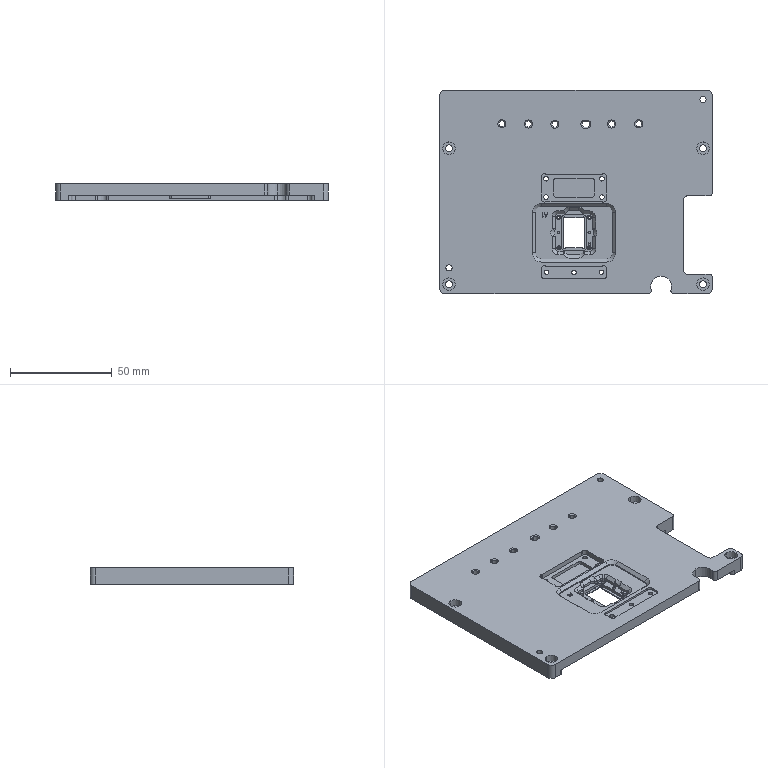NC program | NX | posted with a generic post | part box 134 x 100 x 8 mm
Lines 5752 to 6609 of 16793:
(ZLEVEL_PROFILE_COPY_COPY_COPY_1_COPY_COPY_1_COPY_COPY_COPY_1_COPY_COPY_COPY , )
N11424 T18 M6
N11426 G54
N11428 G17 G0 G90 X-14.95 Y-1.854 S9500 M3
N11430 G43 Z30. H18
N11432 Z-0.177
N11434 G94 G1 X-15.4 Y-2.113 F1000.
N11436 G3 X-15.55 Y-2.373 R0.3
N11438 G1 Y-2.49 F1100.
N11440 G2 X-15.685 Y-3.174 R1.8
N11442 G3 X-15.418 Y-3.432 R0.2
N11444 G2 X-14.802 Y-3.3 R1.5
N11446 G1 X-14.629
N11448 G3 X-14.369 Y-3.15 R0.3
N11450 G1 X-14.109 Y-2.7
N11452 G0 X-14.95 Y-1.854 Z-0.354
N11454 G1 X-15.4 Y-2.113 F1000.
N11456 G3 X-15.55 Y-2.373 R0.3
N11458 G1 Y-2.49 F1100.
N11460 G2 X-15.685 Y-3.174 R1.8
N11462 G3 X-15.418 Y-3.432 R0.2
N11464 G2 X-14.802 Y-3.3 R1.5
N11466 G1 X-14.629
N11468 G3 X-14.369 Y-3.15 R0.3
N11470 G1 X-14.109 Y-2.7
N11472 G0 X-14.95 Y-1.854 Z-0.515
N11474 G1 X-15.4 Y-2.113 F1000.
N11476 G3 X-15.55 Y-2.373 R0.3
N11478 G1 Y-2.49 F1100.
N11480 G2 X-15.685 Y-3.174 R1.8
N11482 G3 X-15.418 Y-3.432 R0.2
N11484 G2 X-14.802 Y-3.3 R1.5
N11486 G1 X-14.629
N11488 G3 X-14.369 Y-3.15 R0.3
N11490 G1 X-14.109 Y-2.7
N11492 G0 X-14.95 Y-1.854 Z-0.677
N11494 G1 X-15.4 Y-2.113 F1000.
N11496 G3 X-15.55 Y-2.373 R0.3
N11498 G1 Y-2.49 F1100.
N11500 G2 X-15.685 Y-3.174 R1.8
N11502 G3 X-15.418 Y-3.432 R0.2
N11504 G2 X-14.802 Y-3.3 R1.5
N11506 G1 X-14.629
N11508 G3 X-14.369 Y-3.15 R0.3
N11510 G1 X-14.109 Y-2.7
N11512 G0 X-14.95 Y-1.854 Z-0.838
N11514 G1 X-15.4 Y-2.113 F1000.
N11516 G3 X-15.55 Y-2.373 R0.3
N11518 G1 Y-2.49 F1100.
N11520 G2 X-15.685 Y-3.174 R1.8
N11522 G3 X-15.418 Y-3.432 R0.2
N11524 G2 X-14.802 Y-3.3 R1.5
N11526 G1 X-14.629
N11528 G3 X-14.369 Y-3.15 R0.3
N11530 G1 X-14.109 Y-2.7
N11532 G0 X-14.95 Y-1.854 Z-1.
N11534 G1 X-15.4 Y-2.113 F1000.
N11536 G3 X-15.55 Y-2.373 R0.3
N11538 G1 Y-2.49 F1100.
N11540 G2 X-15.685 Y-3.174 R1.8
N11542 G3 X-15.418 Y-3.432 R0.2
N11544 G2 X-14.802 Y-3.3 R1.5
N11546 G1 X-14.629
N11548 G3 X-14.369 Y-3.15 R0.3
N11550 G1 X-14.109 Y-2.7
N11552 G0 X-14.95 Y-1.854 Z-1.177
N11554 G1 X-15.4 Y-2.113 F1000.
N11556 G3 X-15.55 Y-2.373 R0.3
N11558 G1 Y-2.49 F1100.
N11560 G2 X-15.685 Y-3.174 R1.8
N11562 G3 X-15.418 Y-3.432 R0.2
N11564 G2 X-14.802 Y-3.3 R1.5
N11566 G1 X-14.629
N11568 G3 X-14.369 Y-3.15 R0.3
N11570 G1 X-14.109 Y-2.7
N11572 G0 X-14.95 Y-1.854 Z-1.354
N11574 G1 X-15.4 Y-2.113 F1000.
N11576 G3 X-15.55 Y-2.373 R0.3
N11578 G1 Y-2.49 F1100.
N11580 G2 X-15.685 Y-3.174 R1.8
N11582 G3 X-15.418 Y-3.432 R0.2
N11584 G2 X-14.802 Y-3.3 R1.5
N11586 G1 X-14.629
N11588 G3 X-14.369 Y-3.15 R0.3
N11590 G1 X-14.109 Y-2.7
N11592 G0 X-14.95 Y-1.854 Z-1.544
N11594 G1 X-15.4 Y-2.113 F1000.
N11596 G3 X-15.55 Y-2.373 R0.3
N11598 G1 Y-2.49 F1100.
N11600 G2 X-15.685 Y-3.174 R1.8
N11602 G3 X-15.418 Y-3.432 R0.2
N11604 G2 X-14.802 Y-3.3 R1.5
N11606 G1 X-14.629
N11608 G3 X-14.369 Y-3.15 R0.3
N11610 G1 X-14.109 Y-2.7
N11612 G0 X-14.95 Y-1.854 Z-1.794
N11614 G1 X-15.4 Y-2.113 F1000.
N11616 G3 X-15.55 Y-2.373 R0.3
N11618 G1 Y-2.49 F1100.
N11620 G2 X-15.685 Y-3.174 R1.8
N11622 G3 X-15.418 Y-3.432 R0.2
N11624 G2 X-14.802 Y-3.3 R1.5
N11626 G1 X-14.629
N11628 G3 X-14.369 Y-3.15 R0.3
N11630 G1 X-14.109 Y-2.7
N11632 G0 X-14.95 Y-1.854 Z-2.
N11634 G1 X-15.4 Y-2.113 F1000.
N11636 G3 X-15.55 Y-2.373 R0.3
N11638 G1 Y-2.49 F1100.
N11640 G2 X-15.685 Y-3.174 R1.8
N11642 G3 X-15.418 Y-3.432 R0.2
N11644 G2 X-14.802 Y-3.3 R1.5
N11646 G1 X-14.629
N11648 G3 X-14.369 Y-3.15 R0.3
N11650 G1 X-14.109 Y-2.7
N11652 G0 X-14.95 Y-1.854 Z-2.1
N11654 G1 X-15.4 Y-2.113 F1000.
N11656 G3 X-15.55 Y-2.373 R0.3
N11658 G1 Y-2.49 F1100.
N11660 G2 X-15.685 Y-3.174 R1.8
N11662 G3 X-15.418 Y-3.432 R0.2
N11664 G2 X-14.802 Y-3.3 R1.5
N11666 G1 X-14.629
N11668 G3 X-14.369 Y-3.15 R0.3
N11670 G1 X-14.109 Y-2.7
N11672 G0 X-14.95 Y-1.854 Z-2.267
N11674 G1 X-15.4 Y-2.113 F1000.
N11676 G3 X-15.55 Y-2.373 R0.3
N11678 G1 Y-2.49 F1100.
N11680 G2 X-15.685 Y-3.174 R1.8
N11682 G3 X-15.418 Y-3.432 R0.2
N11684 G2 X-14.802 Y-3.3 R1.5
N11686 G1 X-14.629
N11688 G3 X-14.369 Y-3.15 R0.3
N11690 G1 X-14.109 Y-2.7
N11692 G0 X-14.95 Y-1.854 Z-2.433
N11694 G1 X-15.4 Y-2.113 F1000.
N11696 G3 X-15.55 Y-2.373 R0.3
N11698 G1 Y-2.49 F1100.
N11700 G2 X-15.685 Y-3.174 R1.8
N11702 G3 X-15.418 Y-3.432 R0.2
N11704 G2 X-14.802 Y-3.3 R1.5
N11706 G1 X-14.629
N11708 G3 X-14.369 Y-3.15 R0.3
N11710 G1 X-14.109 Y-2.7
N11712 G0 X-14.95 Y-1.854 Z-2.6
N11714 G1 X-15.4 Y-2.113 F1000.
N11716 G3 X-15.55 Y-2.373 R0.3
N11718 G1 Y-2.49 F1100.
N11720 G2 X-15.685 Y-3.174 R1.8
N11722 G3 X-15.418 Y-3.432 R0.2
N11724 G2 X-14.802 Y-3.3 R1.5
N11726 G1 X-14.629
N11728 G3 X-14.369 Y-3.15 R0.3
N11730 G1 X-14.109 Y-2.7
N11732 G0 Z30.
N11734 X12.108
N11736 Z-0.177
N11738 G1 X12.368 Y-3.15 F1000.
N11740 G3 X12.627 Y-3.3 R0.3
N11742 G1 X12.74 F1100.
N11744 G2 X13.424 Y-3.435 R1.8
N11746 G3 X13.685 Y-3.174 R0.2
N11748 G2 X13.55 Y-2.49 R1.8
N11750 G1 Y-2.376
N11752 G3 X13.4 Y-2.116 R0.3
N11754 G1 X12.95 Y-1.857
N11756 G0 X12.108 Y-2.7 Z-0.354
N11758 G1 X12.367 Y-3.15 F1000.
N11760 G3 X12.627 Y-3.3 R0.3
N11762 G1 X12.74 F1100.
N11764 G2 X13.424 Y-3.435 R1.8
N11766 G3 X13.685 Y-3.174 R0.2
N11768 G2 X13.55 Y-2.49 R1.8
N11770 G1 Y-2.376
N11772 G3 X13.4 Y-2.116 R0.3
N11774 G1 X12.95 Y-1.856
N11776 G0 X12.108 Y-2.7 Z-0.515
N11778 G1 X12.367 Y-3.15 F1000.
N11780 G3 X12.627 Y-3.3 R0.3
N11782 G1 X12.74 F1100.
N11784 G2 X13.424 Y-3.435 R1.8
N11786 G3 X13.685 Y-3.174 R0.2
N11788 G2 X13.55 Y-2.49 R1.8
N11790 G1 Y-2.375
N11792 G3 X13.4 Y-2.116 R0.3
N11794 G1 X12.95 Y-1.856
N11796 G0 X12.107 Y-2.7 Z-0.677
N11798 G1 X12.367 Y-3.15 F1000.
N11800 G3 X12.627 Y-3.3 R0.3
N11802 G1 X12.74 F1100.
N11804 G2 X13.424 Y-3.435 R1.8
N11806 G3 X13.685 Y-3.174 R0.2
N11808 G2 X13.55 Y-2.49 R1.8
N11810 G1 Y-2.375
N11812 G3 X13.4 Y-2.115 R0.3
N11814 G1 X12.95 Y-1.855
N11816 G0 X12.107 Y-2.7 Z-0.838
N11818 G1 X12.367 Y-3.15 F1000.
N11820 G3 X12.627 Y-3.3 R0.3
N11822 G1 X12.74 F1100.
N11824 G2 X13.424 Y-3.435 R1.8
N11826 G3 X13.685 Y-3.174 R0.2
N11828 G2 X13.55 Y-2.49 R1.8
N11830 G1 Y-2.375
N11832 G3 X13.4 Y-2.115 R0.3
N11834 G1 X12.95 Y-1.855
N11836 G0 X12.107 Y-2.7 Z-1.
N11838 G1 X12.367 Y-3.15 F1000.
N11840 G3 X12.627 Y-3.3 R0.3
N11842 G1 X12.74 F1100.
N11844 G2 X13.424 Y-3.435 R1.8
N11846 G3 X13.685 Y-3.174 R0.2
N11848 G2 X13.55 Y-2.49 R1.8
N11850 G1 Y-2.374
N11852 G3 X13.4 Y-2.114 R0.3
N11854 G1 X12.95 Y-1.855
N11856 G0 X12.107 Y-2.7 Z-1.177
N11858 G1 X12.367 Y-3.15 F1000.
N11860 G3 X12.627 Y-3.3 R0.3
N11862 G1 X12.74 F1100.
N11864 G2 X13.424 Y-3.435 R1.8
N11866 G3 X13.685 Y-3.174 R0.2
N11868 G2 X13.55 Y-2.49 R1.8
N11870 G1 Y-2.374
N11872 G3 X13.4 Y-2.114 R0.3
N11874 G1 X12.95 Y-1.854
N11876 G0 X12.107 Y-2.7 Z-1.354
N11878 G1 X12.367 Y-3.15 F1000.
N11880 G3 X12.627 Y-3.3 R0.3
N11882 G1 X12.74 F1100.
N11884 G2 X13.424 Y-3.435 R1.8
N11886 G3 X13.685 Y-3.174 R0.2
N11888 G2 X13.55 Y-2.49 R1.8
N11890 G1 Y-2.373
N11892 G3 X13.4 Y-2.113 R0.3
N11894 G1 X12.95 Y-1.854
N11896 G0 X12.107 Y-2.7 Z-1.544
N11898 G1 X12.367 Y-3.15 F1000.
N11900 G3 X12.627 Y-3.3 R0.3
N11902 G1 X12.74 F1100.
N11904 G2 X13.424 Y-3.435 R1.8
N11906 G3 X13.685 Y-3.174 R0.2
N11908 G2 X13.55 Y-2.49 R1.8
N11910 G1 Y-2.373
N11912 G3 X13.4 Y-2.113 R0.3
N11914 G1 X12.95 Y-1.853
N11916 G0 X12.107 Y-2.7 Z-1.794
N11918 G1 X12.367 Y-3.15 F1000.
N11920 G3 X12.626 Y-3.3 R0.3
N11922 G1 X12.74 F1100.
N11924 G2 X13.424 Y-3.435 R1.8
N11926 G3 X13.685 Y-3.174 R0.2
N11928 G2 X13.55 Y-2.49 R1.8
N11930 G1 Y-2.372
N11932 G3 X13.4 Y-2.112 R0.3
N11934 G1 X12.95 Y-1.853
N11936 G0 X12.107 Y-2.7 Z-2.
N11938 G1 X12.367 Y-3.15 F1000.
N11940 G3 X12.626 Y-3.3 R0.3
N11942 G1 X12.74 F1100.
N11944 G2 X13.424 Y-3.435 R1.8
N11946 G3 X13.685 Y-3.174 R0.2
N11948 G2 X13.55 Y-2.49 R1.8
N11950 G1 Y-2.372
N11952 G3 X13.4 Y-2.112 R0.3
N11954 G1 X12.95 Y-1.852
N11956 G0 X12.107 Y-2.7 Z-2.1
N11958 G1 X12.366 Y-3.15 F1000.
N11960 G3 X12.626 Y-3.3 R0.3
N11962 G1 X12.74 F1100.
N11964 G2 X13.424 Y-3.435 R1.8
N11966 G3 X13.685 Y-3.174 R0.2
N11968 G2 X13.55 Y-2.49 R1.8
N11970 G1 Y-2.371
N11972 G3 X13.4 Y-2.112 R0.3
N11974 G1 X12.95 Y-1.852
N11976 G0 X12.107 Y-2.7 Z-2.267
N11978 G1 X12.366 Y-3.15 F1000.
N11980 G3 X12.626 Y-3.3 R0.3
N11982 G1 X12.74 F1100.
N11984 G2 X13.424 Y-3.435 R1.8
N11986 G3 X13.685 Y-3.174 R0.2
N11988 G2 X13.55 Y-2.49 R1.8
N11990 G1 Y-2.371
N11992 G3 X13.4 Y-2.111 R0.3
N11994 G1 X12.95 Y-1.851
N11996 G0 X12.106 Y-2.7 Z-2.433
N11998 G1 X12.366 Y-3.15 F1000.
N12000 G3 X12.626 Y-3.3 R0.3
N12002 G1 X12.74 F1100.
N12004 G2 X13.424 Y-3.435 R1.8
N12006 G3 X13.685 Y-3.174 R0.2
N12008 G2 X13.55 Y-2.49 R1.8
N12010 G1 Y-2.371
N12012 G3 X13.4 Y-2.111 R0.3
N12014 G1 X12.95 Y-1.851
N12016 G0 X12.106 Y-2.7 Z-2.6
N12018 G1 X12.366 Y-3.15 F1000.
N12020 G3 X12.626 Y-3.3 R0.3
N12022 G1 X12.74 F1100.
N12024 G2 X13.424 Y-3.435 R1.8
N12026 G3 X13.685 Y-3.174 R0.2
N12028 G2 X13.55 Y-2.49 R1.8
N12030 G1 Y-2.37
N12032 G3 X13.4 Y-2.11 R0.3
N12034 G1 X12.95 Y-1.85
N12036 G0 Z30.
N12038 Y5.858
N12040 Z-0.177
N12042 G1 X13.4 Y6.118 F1000.
N12044 G3 X13.55 Y6.378 R0.3
N12046 G1 Y6.49 F1100.
N12048 G2 X13.685 Y7.174 R1.8
N12050 G3 X13.424 Y7.435 R0.2
N12052 G2 X12.74 Y7.3 R1.8
N12054 G1 X12.628
N12056 G3 X12.368 Y7.15 R0.3
N12058 G1 X12.108 Y6.7
N12060 G0 X12.95 Y5.858 Z-0.354
N12062 G1 X13.4 Y6.118 F1000.
N12064 G3 X13.55 Y6.378 R0.3
N12066 G1 Y6.49 F1100.
N12068 G2 X13.685 Y7.174 R1.8
N12070 G3 X13.424 Y7.435 R0.2
N12072 G2 X12.74 Y7.3 R1.8
N12074 G1 X12.628
N12076 G3 X12.368 Y7.15 R0.3
N12078 G1 X12.108 Y6.7
N12080 G0 X12.95 Y5.858 Z-0.515
N12082 G1 X13.4 Y6.118 F1000.
N12084 G3 X13.55 Y6.378 R0.3
N12086 G1 Y6.49 F1100.
N12088 G2 X13.685 Y7.174 R1.8
N12090 G3 X13.424 Y7.435 R0.2
N12092 G2 X12.74 Y7.3 R1.8
N12094 G1 X12.628
N12096 G3 X12.368 Y7.15 R0.3
N12098 G1 X12.108 Y6.7
N12100 G0 X12.95 Y5.858 Z-0.677
N12102 G1 X13.4 Y6.118 F1000.
N12104 G3 X13.55 Y6.377 R0.3
N12106 G1 Y6.49 F1100.
N12108 G2 X13.685 Y7.174 R1.8
N12110 G3 X13.424 Y7.435 R0.2
N12112 G2 X12.74 Y7.3 R1.8
N12114 G1 X12.627
N12116 G3 X12.368 Y7.15 R0.3
N12118 G1 X12.108 Y6.7
N12120 G0 X12.95 Y5.858 Z-0.838
N12122 G1 X13.4 Y6.118 F1000.
N12124 G3 X13.55 Y6.377 R0.3
N12126 G1 Y6.49 F1100.
N12128 G2 X13.685 Y7.174 R1.8
N12130 G3 X13.424 Y7.435 R0.2
N12132 G2 X12.74 Y7.3 R1.8
N12134 G1 X12.627
N12136 G3 X12.368 Y7.15 R0.3
N12138 G1 X12.108 Y6.7
N12140 G0 X12.95 Y5.858 Z-1.
N12142 G1 X13.4 Y6.118 F1000.
N12144 G3 X13.55 Y6.377 R0.3
N12146 G1 Y6.49 F1100.
N12148 G2 X13.685 Y7.174 R1.8
N12150 G3 X13.424 Y7.435 R0.2
N12152 G2 X12.74 Y7.3 R1.8
N12154 G1 X12.627
N12156 G3 X12.368 Y7.15 R0.3
N12158 G1 X12.108 Y6.7
N12160 G0 X12.95 Y5.858 Z-1.177
N12162 G1 X13.4 Y6.117 F1000.
N12164 G3 X13.55 Y6.377 R0.3
N12166 G1 Y6.49 F1100.
N12168 G2 X13.685 Y7.174 R1.8
N12170 G3 X13.424 Y7.435 R0.2
N12172 G2 X12.74 Y7.3 R1.8
N12174 G1 X12.627
N12176 G3 X12.367 Y7.15 R0.3
N12178 G1 X12.108 Y6.7
N12180 G0 X12.95 Y5.858 Z-1.354
N12182 G1 X13.4 Y6.117 F1000.
N12184 G3 X13.55 Y6.377 R0.3
N12186 G1 Y6.49 F1100.
N12188 G2 X13.685 Y7.174 R1.8
N12190 G3 X13.424 Y7.435 R0.2
N12192 G2 X12.74 Y7.3 R1.8
N12194 G1 X12.627
N12196 G3 X12.367 Y7.15 R0.3
N12198 G1 X12.108 Y6.7
N12200 G0 X12.95 Y5.857 Z-1.544
N12202 G1 X13.4 Y6.117 F1000.
N12204 G3 X13.55 Y6.377 R0.3
N12206 G1 Y6.49 F1100.
N12208 G2 X13.685 Y7.174 R1.8
N12210 G3 X13.424 Y7.435 R0.2
N12212 G2 X12.74 Y7.3 R1.8
N12214 G1 X12.627
N12216 G3 X12.367 Y7.15 R0.3
N12218 G1 X12.107 Y6.7
N12220 G0 X12.95 Y5.857 Z-1.794
N12222 G1 X13.4 Y6.117 F1000.
N12224 G3 X13.55 Y6.377 R0.3
N12226 G1 Y6.49 F1100.
N12228 G2 X13.685 Y7.174 R1.8
N12230 G3 X13.424 Y7.435 R0.2
N12232 G2 X12.74 Y7.3 R1.8
N12234 G1 X12.627
N12236 G3 X12.367 Y7.15 R0.3
N12238 G1 X12.107 Y6.7
N12240 G0 X12.95 Y5.857 Z-2.
N12242 G1 X13.4 Y6.117 F1000.
N12244 G3 X13.55 Y6.377 R0.3
N12246 G1 Y6.49 F1100.
N12248 G2 X13.685 Y7.174 R1.8
N12250 G3 X13.424 Y7.435 R0.2
N12252 G2 X12.74 Y7.3 R1.8
N12254 G1 X12.627
N12256 G3 X12.367 Y7.15 R0.3
N12258 G1 X12.107 Y6.7
N12260 G0 X12.95 Y5.857 Z-2.1
N12262 G1 X13.4 Y6.117 F1000.
N12264 G3 X13.55 Y6.377 R0.3
N12266 G1 Y6.49 F1100.
N12268 G2 X13.685 Y7.174 R1.8
N12270 G3 X13.424 Y7.435 R0.2
N12272 G2 X12.74 Y7.3 R1.8
N12274 G1 X12.627
N12276 G3 X12.367 Y7.15 R0.3
N12278 G1 X12.107 Y6.7
N12280 G0 X12.95 Y5.857 Z-2.267
N12282 G1 X13.4 Y6.117 F1000.
N12284 G3 X13.55 Y6.377 R0.3
N12286 G1 Y6.49 F1100.
N12288 G2 X13.685 Y7.174 R1.8
N12290 G3 X13.424 Y7.435 R0.2
N12292 G2 X12.74 Y7.3 R1.8
N12294 G1 X12.627
N12296 G3 X12.367 Y7.15 R0.3
N12298 G1 X12.107 Y6.7
N12300 G0 X12.95 Y5.857 Z-2.433
N12302 G1 X13.4 Y6.117 F1000.
N12304 G3 X13.55 Y6.377 R0.3
N12306 G1 Y6.49 F1100.
N12308 G2 X13.685 Y7.174 R1.8
N12310 G3 X13.424 Y7.435 R0.2
N12312 G2 X12.74 Y7.3 R1.8
N12314 G1 X12.627
N12316 G3 X12.367 Y7.15 R0.3
N12318 G1 X12.107 Y6.7
N12320 G0 X12.95 Y5.857 Z-2.6
N12322 G1 X13.4 Y6.117 F1000.
N12324 G3 X13.55 Y6.377 R0.3
N12326 G1 Y6.49 F1100.
N12328 G2 X13.685 Y7.174 R1.8
N12330 G3 X13.424 Y7.435 R0.2
N12332 G2 X12.74 Y7.3 R1.8
N12334 G1 X12.627
N12336 G3 X12.367 Y7.15 R0.3
N12338 G1 X12.107 Y6.7
N12340 G0 Z30.
N12342 X-14.108
N12344 Z-0.177
N12346 G1 X-14.368 Y7.15 F1000.
N12348 G3 X-14.628 Y7.3 R0.3
N12350 G1 X-14.74 F1100.
N12352 G2 X-15.424 Y7.435 R1.8
N12354 G3 X-15.685 Y7.174 R0.2
N12356 G2 X-15.55 Y6.49 R1.8
N12358 G1 Y6.378
N12360 G3 X-15.4 Y6.118 R0.3
N12362 G1 X-14.95 Y5.858
N12364 G0 X-14.108 Y6.7 Z-0.354
N12366 G1 X-14.368 Y7.15 F1000.
N12368 G3 X-14.628 Y7.3 R0.3
N12370 G1 X-14.74 F1100.
N12372 G2 X-15.424 Y7.435 R1.8
N12374 G3 X-15.685 Y7.174 R0.2
N12376 G2 X-15.55 Y6.49 R1.8
N12378 G1 Y6.378
N12380 G3 X-15.4 Y6.118 R0.3
N12382 G1 X-14.95 Y5.858
N12384 G0 X-14.108 Y6.7 Z-0.515
N12386 G1 X-14.368 Y7.15 F1000.
N12388 G3 X-14.628 Y7.3 R0.3
N12390 G1 X-14.74 F1100.
N12392 G2 X-15.424 Y7.435 R1.8
N12394 G3 X-15.685 Y7.174 R0.2
N12396 G2 X-15.55 Y6.49 R1.8
N12398 G1 Y6.378
N12400 G3 X-15.4 Y6.118 R0.3
N12402 G1 X-14.95 Y5.858
N12404 G0 X-14.108 Y6.7 Z-0.677
N12406 G1 X-14.368 Y7.15 F1000.
N12408 G3 X-14.628 Y7.3 R0.3
N12410 G1 X-14.74 F1100.
N12412 G2 X-15.424 Y7.435 R1.8
N12414 G3 X-15.685 Y7.174 R0.2
N12416 G2 X-15.55 Y6.49 R1.8
N12418 G1 Y6.378
N12420 G3 X-15.4 Y6.118 R0.3
N12422 G1 X-14.95 Y5.858
N12424 G0 X-14.108 Y6.7 Z-0.838
N12426 G1 X-14.368 Y7.15 F1000.
N12428 G3 X-14.628 Y7.3 R0.3
N12430 G1 X-14.74 F1100.
N12432 G2 X-15.424 Y7.435 R1.8
N12434 G3 X-15.685 Y7.174 R0.2
N12436 G2 X-15.55 Y6.49 R1.8
N12438 G1 Y6.378
N12440 G3 X-15.4 Y6.118 R0.3
N12442 G1 X-14.95 Y5.858
N12444 G0 X-14.108 Y6.7 Z-1.
N12446 G1 X-14.368 Y7.15 F1000.
N12448 G3 X-14.628 Y7.3 R0.3
N12450 G1 X-14.74 F1100.
N12452 G2 X-15.424 Y7.435 R1.8
N12454 G3 X-15.685 Y7.174 R0.2
N12456 G2 X-15.55 Y6.49 R1.8
N12458 G1 Y6.378
N12460 G3 X-15.4 Y6.118 R0.3
N12462 G1 X-14.95 Y5.858
N12464 G0 X-14.108 Y6.7 Z-1.177
N12466 G1 X-14.368 Y7.15 F1000.
N12468 G3 X-14.628 Y7.3 R0.3
N12470 G1 X-14.74 F1100.
N12472 G2 X-15.424 Y7.435 R1.8
N12474 G3 X-15.685 Y7.174 R0.2
N12476 G2 X-15.55 Y6.49 R1.8
N12478 G1 Y6.378
N12480 G3 X-15.4 Y6.118 R0.3
N12482 G1 X-14.95 Y5.858
N12484 G0 X-14.108 Y6.7 Z-1.354
N12486 G1 X-14.368 Y7.15 F1000.
N12488 G3 X-14.628 Y7.3 R0.3
N12490 G1 X-14.74 F1100.
N12492 G2 X-15.424 Y7.435 R1.8
N12494 G3 X-15.685 Y7.174 R0.2
N12496 G2 X-15.55 Y6.49 R1.8
N12498 G1 Y6.378
N12500 G3 X-15.4 Y6.118 R0.3
N12502 G1 X-14.95 Y5.858
N12504 G0 X-14.108 Y6.7 Z-1.544
N12506 G1 X-14.368 Y7.15 F1000.
N12508 G3 X-14.628 Y7.3 R0.3
N12510 G1 X-14.74 F1100.
N12512 G2 X-15.424 Y7.435 R1.8
N12514 G3 X-15.685 Y7.174 R0.2
N12516 G2 X-15.55 Y6.49 R1.8
N12518 G1 Y6.378
N12520 G3 X-15.4 Y6.118 R0.3
N12522 G1 X-14.95 Y5.858
N12524 G0 X-14.108 Y6.7 Z-1.794
N12526 G1 X-14.368 Y7.15 F1000.
N12528 G3 X-14.628 Y7.3 R0.3
N12530 G1 X-14.74 F1100.
N12532 G2 X-15.424 Y7.435 R1.8
N12534 G3 X-15.685 Y7.174 R0.2
N12536 G2 X-15.55 Y6.49 R1.8
N12538 G1 Y6.378
N12540 G3 X-15.4 Y6.118 R0.3
N12542 G1 X-14.95 Y5.858
N12544 G0 X-14.108 Y6.7 Z-2.
N12546 G1 X-14.368 Y7.15 F1000.
N12548 G3 X-14.628 Y7.3 R0.3
N12550 G1 X-14.74 F1100.
N12552 G2 X-15.424 Y7.435 R1.8
N12554 G3 X-15.685 Y7.174 R0.2
N12556 G2 X-15.55 Y6.49 R1.8
N12558 G1 Y6.378
N12560 G3 X-15.4 Y6.118 R0.3
N12562 G1 X-14.95 Y5.858
N12564 G0 X-14.108 Y6.7 Z-2.1
N12566 G1 X-14.368 Y7.15 F1000.
N12568 G3 X-14.628 Y7.3 R0.3
N12570 G1 X-14.74 F1100.
N12572 G2 X-15.424 Y7.435 R1.8
N12574 G3 X-15.685 Y7.174 R0.2
N12576 G2 X-15.55 Y6.49 R1.8
N12578 G1 Y6.378
N12580 G3 X-15.4 Y6.118 R0.3
N12582 G1 X-14.95 Y5.858
N12584 G0 X-14.108 Y6.7 Z-2.267
N12586 G1 X-14.368 Y7.15 F1000.
N12588 G3 X-14.628 Y7.3 R0.3
N12590 G1 X-14.74 F1100.
N12592 G2 X-15.424 Y7.435 R1.8
N12594 G3 X-15.685 Y7.174 R0.2
N12596 G2 X-15.55 Y6.49 R1.8
N12598 G1 Y6.378
N12600 G3 X-15.4 Y6.118 R0.3
N12602 G1 X-14.95 Y5.858
N12604 G0 X-14.108 Y6.7 Z-2.433
N12606 G1 X-14.368 Y7.15 F1000.
N12608 G3 X-14.628 Y7.3 R0.3
N12610 G1 X-14.74 F1100.
N12612 G2 X-15.424 Y7.435 R1.8
N12614 G3 X-15.685 Y7.174 R0.2
N12616 G2 X-15.55 Y6.49 R1.8
N12618 G1 Y6.378
N12620 G3 X-15.4 Y6.118 R0.3
N12622 G1 X-14.95 Y5.858
N12624 G0 X-14.108 Y6.7 Z-2.6
N12626 G1 X-14.368 Y7.15 F1000.
N12628 G3 X-14.628 Y7.3 R0.3
N12630 G1 X-14.74 F1100.
N12632 G2 X-15.424 Y7.435 R1.8
N12634 G3 X-15.685 Y7.174 R0.2
N12636 G2 X-15.55 Y6.49 R1.8
N12638 G1 Y6.378
N12640 G3 X-15.4 Y6.118 R0.3
N12642 G1 X-14.95 Y5.858
N12644 G0 Z30.
N12646 Y-39.608
N12648 Z-0.177
N12650 G1 X-15.4 Y-39.868 F1000.
N12652 G3 X-15.55 Y-40.128 R0.3
N12654 G1 Y-40.24 F1100.
N12656 G2 X-15.685 Y-40.924 R1.8
N12658 G3 X-15.424 Y-41.185 R0.2
N12660 G2 X-14.74 Y-41.05 R1.8
N12662 G1 X-14.628
N12664 G3 X-14.368 Y-40.9 R0.3
N12666 G1 X-14.108 Y-40.45
N12668 G0 X-14.95 Y-39.608 Z-0.354
N12670 G1 X-15.4 Y-39.868 F1000.
N12672 G3 X-15.55 Y-40.128 R0.3
N12674 G1 Y-40.24 F1100.
N12676 G2 X-15.685 Y-40.924 R1.8
N12678 G3 X-15.424 Y-41.185 R0.2
N12680 G2 X-14.74 Y-41.05 R1.8
N12682 G1 X-14.628
N12684 G3 X-14.368 Y-40.9 R0.3
N12686 G1 X-14.108 Y-40.45
N12688 G0 X-14.95 Y-39.608 Z-0.515
N12690 G1 X-15.4 Y-39.868 F1000.
N12692 G3 X-15.55 Y-40.128 R0.3
N12694 G1 Y-40.24 F1100.
N12696 G2 X-15.685 Y-40.924 R1.8
N12698 G3 X-15.424 Y-41.185 R0.2
N12700 G2 X-14.74 Y-41.05 R1.8
N12702 G1 X-14.628
N12704 G3 X-14.368 Y-40.9 R0.3
N12706 G1 X-14.108 Y-40.45
N12708 G0 X-14.95 Y-39.608 Z-0.677
N12710 G1 X-15.4 Y-39.868 F1000.
N12712 G3 X-15.55 Y-40.128 R0.3
N12714 G1 Y-40.24 F1100.
N12716 G2 X-15.685 Y-40.924 R1.8
N12718 G3 X-15.424 Y-41.185 R0.2
N12720 G2 X-14.74 Y-41.05 R1.8
N12722 G1 X-14.628
N12724 G3 X-14.368 Y-40.9 R0.3
N12726 G1 X-14.108 Y-40.45
N12728 G0 X-14.95 Y-39.608 Z-0.838
N12730 G1 X-15.4 Y-39.868 F1000.
N12732 G3 X-15.55 Y-40.128 R0.3
N12734 G1 Y-40.24 F1100.
N12736 G2 X-15.685 Y-40.924 R1.8
N12738 G3 X-15.424 Y-41.185 R0.2
N12740 G2 X-14.74 Y-41.05 R1.8
N12742 G1 X-14.628
N12744 G3 X-14.368 Y-40.9 R0.3
N12746 G1 X-14.108 Y-40.45
N12748 G0 X-14.95 Y-39.608 Z-1.
N12750 G1 X-15.4 Y-39.868 F1000.
N12752 G3 X-15.55 Y-40.127 R0.3
N12754 G1 Y-40.24 F1100.
N12756 G2 X-15.685 Y-40.924 R1.8
N12758 G3 X-15.424 Y-41.185 R0.2
N12760 G2 X-14.74 Y-41.05 R1.8
N12762 G1 X-14.627
N12764 G3 X-14.368 Y-40.9 R0.3
N12766 G1 X-14.108 Y-40.45
N12768 G0 Z30.
N12770 X12.108
N12772 Z-0.177
N12774 G1 X12.368 Y-40.9 F1000.
N12776 G3 X12.628 Y-41.05 R0.3
N12778 G1 X12.74 F1100.
N12780 G2 X13.424 Y-41.185 R1.8
N12782 G3 X13.685 Y-40.924 R0.2
N12784 G2 X13.55 Y-40.24 R1.8
N12786 G1 Y-40.128
N12788 G3 X13.4 Y-39.868 R0.3
N12790 G1 X12.95 Y-39.608
N12792 G0 X12.108 Y-40.45 Z-0.354
N12794 G1 X12.368 Y-40.9 F1000.
N12796 G3 X12.628 Y-41.05 R0.3
N12798 G1 X12.74 F1100.
N12800 G2 X13.424 Y-41.185 R1.8
N12802 G3 X13.685 Y-40.924 R0.2
N12804 G2 X13.55 Y-40.24 R1.8
N12806 G1 Y-40.128
N12808 G3 X13.4 Y-39.868 R0.3
N12810 G1 X12.95 Y-39.608
N12812 G0 X12.108 Y-40.45 Z-0.515
N12814 G1 X12.368 Y-40.9 F1000.
N12816 G3 X12.628 Y-41.05 R0.3
N12818 G1 X12.74 F1100.
N12820 G2 X13.424 Y-41.185 R1.8
N12822 G3 X13.685 Y-40.924 R0.2
N12824 G2 X13.55 Y-40.24 R1.8
N12826 G1 Y-40.128
N12828 G3 X13.4 Y-39.868 R0.3
N12830 G1 X12.95 Y-39.608
N12832 G0 X12.108 Y-40.45 Z-0.677
N12834 G1 X12.368 Y-40.9 F1000.
N12836 G3 X12.628 Y-41.05 R0.3
N12838 G1 X12.74 F1100.
N12840 G2 X13.424 Y-41.185 R1.8
N12842 G3 X13.685 Y-40.924 R0.2
N12844 G2 X13.55 Y-40.24 R1.8
N12846 G1 Y-40.128
N12848 G3 X13.4 Y-39.868 R0.3
N12850 G1 X12.95 Y-39.608
N12852 G0 X12.108 Y-40.45 Z-0.838
N12854 G1 X12.368 Y-40.9 F1000.
N12856 G3 X12.628 Y-41.05 R0.3
N12858 G1 X12.74 F1100.
N12860 G2 X13.424 Y-41.185 R1.8
N12862 G3 X13.685 Y-40.924 R0.2
N12864 G2 X13.55 Y-40.24 R1.8
N12866 G1 Y-40.128
N12868 G3 X13.4 Y-39.868 R0.3
N12870 G1 X12.95 Y-39.608
N12872 G0 X12.108 Y-40.45 Z-1.
N12874 G1 X12.368 Y-40.9 F1000.
N12876 G3 X12.628 Y-41.05 R0.3
N12878 G1 X12.74 F1100.
N12880 G2 X13.424 Y-41.185 R1.8
N12882 G3 X13.685 Y-40.924 R0.2
N12884 G2 X13.55 Y-40.24 R1.8
N12886 G1 Y-40.128
N12888 G3 X13.4 Y-39.868 R0.3
N12890 G1 X12.95 Y-39.608
N12892 G0 Z30.
N12894 Y-39.392
N12896 Z-0.177
N12898 G1 X13.4 Y-39.132 F1000.
N12900 G3 X13.55 Y-38.872 R0.3
N12902 G1 Y-38.76 F1100.
N12904 G2 X13.685 Y-38.076 R1.8
N12906 G3 X13.424 Y-37.815 R0.2
N12908 G2 X12.74 Y-37.95 R1.8
N12910 G1 X12.628
N12912 G3 X12.368 Y-38.1 R0.3
N12914 G1 X12.108 Y-38.55
N12916 G0 X12.95 Y-39.392 Z-0.354
N12918 G1 X13.4 Y-39.132 F1000.
N12920 G3 X13.55 Y-38.872 R0.3
N12922 G1 Y-38.76 F1100.
N12924 G2 X13.685 Y-38.076 R1.8
N12926 G3 X13.424 Y-37.815 R0.2
N12928 G2 X12.74 Y-37.95 R1.8
N12930 G1 X12.628
N12932 G3 X12.368 Y-38.1 R0.3
N12934 G1 X12.108 Y-38.55
N12936 G0 X12.95 Y-39.392 Z-0.515
N12938 G1 X13.4 Y-39.132 F1000.
N12940 G3 X13.55 Y-38.872 R0.3
N12942 G1 Y-38.76 F1100.
N12944 G2 X13.685 Y-38.076 R1.8
N12946 G3 X13.424 Y-37.815 R0.2
N12948 G2 X12.74 Y-37.95 R1.8
N12950 G1 X12.628
N12952 G3 X12.368 Y-38.1 R0.3
N12954 G1 X12.108 Y-38.55
N12956 G0 X12.95 Y-39.392 Z-0.677
N12958 G1 X13.4 Y-39.132 F1000.
N12960 G3 X13.55 Y-38.872 R0.3
N12962 G1 Y-38.76 F1100.
N12964 G2 X13.685 Y-38.076 R1.8
N12966 G3 X13.424 Y-37.815 R0.2
N12968 G2 X12.74 Y-37.95 R1.8
N12970 G1 X12.628
N12972 G3 X12.368 Y-38.1 R0.3
N12974 G1 X12.108 Y-38.55
N12976 G0 X12.95 Y-39.392 Z-0.838
N12978 G1 X13.4 Y-39.132 F1000.
N12980 G3 X13.55 Y-38.872 R0.3
N12982 G1 Y-38.76 F1100.
N12984 G2 X13.685 Y-38.076 R1.8
N12986 G3 X13.424 Y-37.815 R0.2
N12988 G2 X12.74 Y-37.95 R1.8
N12990 G1 X12.628
N12992 G3 X12.368 Y-38.1 R0.3
N12994 G1 X12.108 Y-38.55
N12996 G0 X12.95 Y-39.392 Z-1.
N12998 G1 X13.4 Y-39.132 F1000.
N13000 G3 X13.55 Y-38.872 R0.3
N13002 G1 Y-38.76 F1100.
N13004 G2 X13.685 Y-38.076 R1.8
N13006 G3 X13.424 Y-37.815 R0.2
N13008 G2 X12.74 Y-37.95 R1.8
N13010 G1 X12.628
N13012 G3 X12.368 Y-38.1 R0.3
N13014 G1 X12.108 Y-38.55
N13016 G0 Z30.
N13018 X-14.108
N13020 Z-0.177
N13022 G1 X-14.368 Y-38.1 F1000.
N13024 G3 X-14.628 Y-37.95 R0.3
N13026 G1 X-14.74 F1100.
N13028 G2 X-15.424 Y-37.815 R1.8
N13030 G3 X-15.685 Y-38.076 R0.2
N13032 G2 X-15.55 Y-38.76 R1.8
N13034 G1 Y-38.872
N13036 G3 X-15.4 Y-39.132 R0.3
N13038 G1 X-14.95 Y-39.392
N13040 G0 X-14.108 Y-38.55 Z-0.354
N13042 G1 X-14.368 Y-38.1 F1000.
N13044 G3 X-14.628 Y-37.95 R0.3
N13046 G1 X-14.74 F1100.
N13048 G2 X-15.424 Y-37.815 R1.8
N13050 G3 X-15.685 Y-38.076 R0.2
N13052 G2 X-15.55 Y-38.76 R1.8
N13054 G1 Y-38.872
N13056 G3 X-15.4 Y-39.132 R0.3
N13058 G1 X-14.95 Y-39.392
N13060 G0 X-14.108 Y-38.55 Z-0.515
N13062 G1 X-14.368 Y-38.1 F1000.
N13064 G3 X-14.628 Y-37.95 R0.3
N13066 G1 X-14.74 F1100.
N13068 G2 X-15.424 Y-37.815 R1.8
N13070 G3 X-15.685 Y-38.076 R0.2
N13072 G2 X-15.55 Y-38.76 R1.8
N13074 G1 Y-38.872
N13076 G3 X-15.4 Y-39.132 R0.3
N13078 G1 X-14.95 Y-39.392
N13080 G0 X-14.108 Y-38.55 Z-0.677
N13082 G1 X-14.368 Y-38.1 F1000.
N13084 G3 X-14.628 Y-37.95 R0.3
N13086 G1 X-14.74 F1100.
N13088 G2 X-15.424 Y-37.815 R1.8
N13090 G3 X-15.685 Y-38.076 R0.2
N13092 G2 X-15.55 Y-38.76 R1.8
N13094 G1 Y-38.872
N13096 G3 X-15.4 Y-39.132 R0.3
N13098 G1 X-14.95 Y-39.392
N13100 G0 X-14.108 Y-38.55 Z-0.838
N13102 G1 X-14.368 Y-38.1 F1000.
N13104 G3 X-14.628 Y-37.95 R0.3
N13106 G1 X-14.74 F1100.
N13108 G2 X-15.424 Y-37.815 R1.8
N13110 G3 X-15.685 Y-38.076 R0.2
N13112 G2 X-15.55 Y-38.76 R1.8
N13114 G1 Y-38.872
N13116 G3 X-15.4 Y-39.132 R0.3
N13118 G1 X-14.95 Y-39.392
N13120 G0 X-14.108 Y-38.55 Z-1.
N13122 G1 X-14.368 Y-38.1 F1000.
N13124 G3 X-14.628 Y-37.95 R0.3
N13126 G1 X-14.74 F1100.
N13128 G2 X-15.424 Y-37.815 R1.8
N13130 G3 X-15.685 Y-38.076 R0.2
N13132 G2 X-15.55 Y-38.76 R1.8